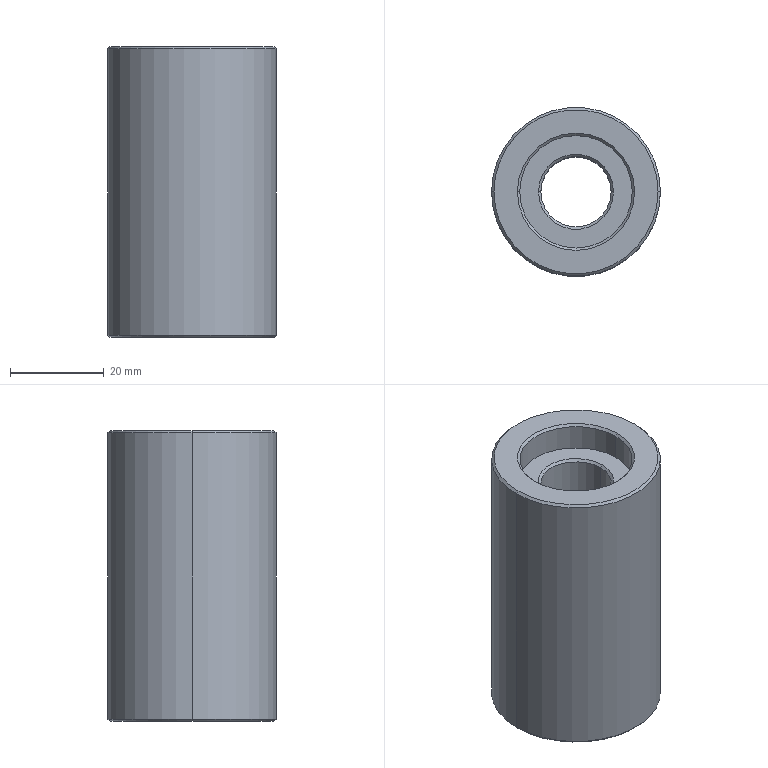Part | STEP file | 1 solid | 24 faces | box 36 x 36 x 62 mm | volume 48785 mm3 | cone 12 | cylinder 8 | plane 4 | commonest cylinder face diameters 24 x4 15 x2 36 x2
STEP:
#1=CARTESIAN_POINT('',(0.,0.,0.));
#2=DIRECTION('',(0.,0.,1.));
#3=DIRECTION('',(1.,0.,0.));
#4=AXIS2_PLACEMENT_3D('',#1,#2,#3);
#5=CARTESIAN_POINT('',(7.5,0.,55.5));
#6=VERTEX_POINT('',#5);
#7=CARTESIAN_POINT('',(8.,0.,56.));
#8=VERTEX_POINT('',#7);
#9=CARTESIAN_POINT('',(7.5,0.,55.5));
#10=DIRECTION('',(0.7071,0.,0.7071));
#11=VECTOR('',#10,1.);
#12=LINE('',#9,#11);
#13=CARTESIAN_POINT('',(0.,0.,55.5));
#14=DIRECTION('',(0.,0.,1.));
#15=DIRECTION('',(1.,0.,0.));
#16=AXIS2_PLACEMENT_3D('',#13,#14,#15);
#17=CONICAL_SURFACE('',#16,7.5,0.7854);
#18=CARTESIAN_POINT('',(6.283,0.));
#19=DIRECTION('',(0.,1.));
#20=VECTOR('',#19,1.);
#21=LINE('',#18,#20);
#22=(GEOMETRIC_REPRESENTATION_CONTEXT(2)PARAMETRIC_REPRESENTATION_CONTEXT()REPRESENTATION_CONTEXT('',''));
#23=DEFINITIONAL_REPRESENTATION('',(#21),#22);
#24=PCURVE('',#17,#23);
#25=CARTESIAN_POINT('',(0.,0.,55.5));
#26=DIRECTION('',(0.,0.,1.));
#27=DIRECTION('',(1.,0.,0.));
#28=AXIS2_PLACEMENT_3D('',#25,#26,#27);
#29=CONICAL_SURFACE('',#28,7.5,0.7854);
#30=CARTESIAN_POINT('',(0.,0.));
#31=DIRECTION('',(0.,1.));
#32=VECTOR('',#31,1.);
#33=LINE('',#30,#32);
#34=(GEOMETRIC_REPRESENTATION_CONTEXT(2)PARAMETRIC_REPRESENTATION_CONTEXT()REPRESENTATION_CONTEXT('',''));
#35=DEFINITIONAL_REPRESENTATION('',(#33),#34);
#36=PCURVE('',#29,#35);
#37=SURFACE_CURVE('',#12,(#24,#36),.PCURVE_S1.);
#38=EDGE_CURVE('',#6,#8,#37,.T.);
#39=ORIENTED_EDGE('',*,*,#38,.T.);
#40=CARTESIAN_POINT('',(-8.,0.,56.));
#41=VERTEX_POINT('',#40);
#42=CARTESIAN_POINT('',(0.,0.,56.));
#43=DIRECTION('',(0.,0.,-1.));
#44=DIRECTION('',(1.,0.,0.));
#45=AXIS2_PLACEMENT_3D('',#42,#43,#44);
#46=CIRCLE('',#45,8.);
#47=CARTESIAN_POINT('',(6.283,0.5));
#48=DIRECTION('',(-1.,0.));
#49=VECTOR('',#48,1.);
#50=LINE('',#47,#49);
#51=(GEOMETRIC_REPRESENTATION_CONTEXT(2)PARAMETRIC_REPRESENTATION_CONTEXT()REPRESENTATION_CONTEXT('',''));
#52=DEFINITIONAL_REPRESENTATION('',(#50),#51);
#53=PCURVE('',#17,#52);
#54=CARTESIAN_POINT('',(0.,0.,56.));
#55=DIRECTION('',(0.,0.,1.));
#56=DIRECTION('',(1.,0.,0.));
#57=AXIS2_PLACEMENT_3D('',#54,#55,#56);
#58=PLANE('',#57);
#59=CARTESIAN_POINT('',(8.,0.));
#60=CARTESIAN_POINT('',(8.,-13.856));
#61=CARTESIAN_POINT('',(-4.,-6.928));
#62=CARTESIAN_POINT('',(-16.,0.));
#63=CARTESIAN_POINT('',(-4.,6.928));
#64=CARTESIAN_POINT('',(8.,13.856));
#65=CARTESIAN_POINT('',(8.,0.));
#66=(BOUNDED_CURVE()B_SPLINE_CURVE(2,(#59,#60,#61,#62,#63,#64,#65),.UNSPECIFIED.,.T.,.F.)B_SPLINE_CURVE_WITH_KNOTS((1,2,2,2,2,1),(-2.094,0.,2.094,4.189,6.283,8.378),.UNSPECIFIED.)CURVE()GEOMETRIC_REPRESENTATION_ITEM()RATIONAL_B_SPLINE_CURVE((1.,0.5,1.,0.5,1.,0.5,1.))REPRESENTATION_ITEM(''));
#67=(GEOMETRIC_REPRESENTATION_CONTEXT(2)PARAMETRIC_REPRESENTATION_CONTEXT()REPRESENTATION_CONTEXT('',''));
#68=DEFINITIONAL_REPRESENTATION('',(#66),#67);
#69=PCURVE('',#58,#68);
#70=SURFACE_CURVE('',#46,(#53,#69),.PCURVE_S1.);
#71=EDGE_CURVE('',#8,#41,#70,.T.);
#72=ORIENTED_EDGE('',*,*,#71,.T.);
#73=CARTESIAN_POINT('',(-7.5,0.,55.5));
#74=VERTEX_POINT('',#73);
#75=CARTESIAN_POINT('',(-7.5,0.,55.5));
#76=DIRECTION('',(-0.7071,0.,0.7071));
#77=VECTOR('',#76,1.);
#78=LINE('',#75,#77);
#79=CARTESIAN_POINT('',(3.142,0.));
#80=DIRECTION('',(0.,1.));
#81=VECTOR('',#80,1.);
#82=LINE('',#79,#81);
#83=(GEOMETRIC_REPRESENTATION_CONTEXT(2)PARAMETRIC_REPRESENTATION_CONTEXT()REPRESENTATION_CONTEXT('',''));
#84=DEFINITIONAL_REPRESENTATION('',(#82),#83);
#85=PCURVE('',#17,#84);
#86=CARTESIAN_POINT('',(3.142,0.));
#87=DIRECTION('',(0.,1.));
#88=VECTOR('',#87,1.);
#89=LINE('',#86,#88);
#90=(GEOMETRIC_REPRESENTATION_CONTEXT(2)PARAMETRIC_REPRESENTATION_CONTEXT()REPRESENTATION_CONTEXT('',''));
#91=DEFINITIONAL_REPRESENTATION('',(#89),#90);
#92=PCURVE('',#29,#91);
#93=SURFACE_CURVE('',#78,(#85,#92),.PCURVE_S1.);
#94=EDGE_CURVE('',#74,#41,#93,.T.);
#95=ORIENTED_EDGE('',*,*,#94,.F.);
#96=CARTESIAN_POINT('',(0.,0.,55.5));
#97=DIRECTION('',(0.,0.,1.));
#98=DIRECTION('',(1.,0.,0.));
#99=AXIS2_PLACEMENT_3D('',#96,#97,#98);
#100=CIRCLE('',#99,7.5);
#101=CARTESIAN_POINT('',(0.,0.));
#102=DIRECTION('',(1.,0.));
#103=VECTOR('',#102,1.);
#104=LINE('',#101,#103);
#105=(GEOMETRIC_REPRESENTATION_CONTEXT(2)PARAMETRIC_REPRESENTATION_CONTEXT()REPRESENTATION_CONTEXT('',''));
#106=DEFINITIONAL_REPRESENTATION('',(#104),#105);
#107=PCURVE('',#17,#106);
#108=CARTESIAN_POINT('',(0.,0.,62.));
#109=DIRECTION('',(0.,0.,-1.));
#110=DIRECTION('',(-1.,0.,0.));
#111=AXIS2_PLACEMENT_3D('',#108,#109,#110);
#112=CYLINDRICAL_SURFACE('',#111,7.5);
#113=CARTESIAN_POINT('',(9.425,6.5));
#114=DIRECTION('',(-1.,0.));
#115=VECTOR('',#114,1.);
#116=LINE('',#113,#115);
#117=(GEOMETRIC_REPRESENTATION_CONTEXT(2)PARAMETRIC_REPRESENTATION_CONTEXT()REPRESENTATION_CONTEXT('',''));
#118=DEFINITIONAL_REPRESENTATION('',(#116),#117);
#119=PCURVE('',#112,#118);
#120=SURFACE_CURVE('',#100,(#107,#119),.PCURVE_S1.);
#121=EDGE_CURVE('',#74,#6,#120,.T.);
#122=ORIENTED_EDGE('',*,*,#121,.T.);
#123=EDGE_LOOP('',(#39,#72,#95,#122));
#124=FACE_BOUND('',#123,.F.);
#125=ADVANCED_FACE('',(#124),#17,.F.);
#126=CARTESIAN_POINT('',(12.,0.,61.5));
#127=VERTEX_POINT('',#126);
#128=CARTESIAN_POINT('',(12.5,0.,62.));
#129=VERTEX_POINT('',#128);
#130=CARTESIAN_POINT('',(12.,0.,61.5));
#131=DIRECTION('',(0.7071,0.,0.7071));
#132=VECTOR('',#131,1.);
#133=LINE('',#130,#132);
#134=CARTESIAN_POINT('',(0.,0.,61.5));
#135=DIRECTION('',(0.,0.,1.));
#136=DIRECTION('',(1.,0.,0.));
#137=AXIS2_PLACEMENT_3D('',#134,#135,#136);
#138=CONICAL_SURFACE('',#137,12.,0.7854);
#139=CARTESIAN_POINT('',(6.283,0.));
#140=DIRECTION('',(0.,1.));
#141=VECTOR('',#140,1.);
#142=LINE('',#139,#141);
#143=(GEOMETRIC_REPRESENTATION_CONTEXT(2)PARAMETRIC_REPRESENTATION_CONTEXT()REPRESENTATION_CONTEXT('',''));
#144=DEFINITIONAL_REPRESENTATION('',(#142),#143);
#145=PCURVE('',#138,#144);
#146=CARTESIAN_POINT('',(0.,0.,61.5));
#147=DIRECTION('',(0.,0.,1.));
#148=DIRECTION('',(1.,0.,0.));
#149=AXIS2_PLACEMENT_3D('',#146,#147,#148);
#150=CONICAL_SURFACE('',#149,12.,0.7854);
#151=CARTESIAN_POINT('',(0.,0.));
#152=DIRECTION('',(0.,1.));
#153=VECTOR('',#152,1.);
#154=LINE('',#151,#153);
#155=(GEOMETRIC_REPRESENTATION_CONTEXT(2)PARAMETRIC_REPRESENTATION_CONTEXT()REPRESENTATION_CONTEXT('',''));
#156=DEFINITIONAL_REPRESENTATION('',(#154),#155);
#157=PCURVE('',#150,#156);
#158=SURFACE_CURVE('',#133,(#145,#157),.PCURVE_S1.);
#159=EDGE_CURVE('',#127,#129,#158,.T.);
#160=ORIENTED_EDGE('',*,*,#159,.T.);
#161=CARTESIAN_POINT('',(-12.5,0.,62.));
#162=VERTEX_POINT('',#161);
#163=CARTESIAN_POINT('',(0.,0.,62.));
#164=DIRECTION('',(0.,0.,-1.));
#165=DIRECTION('',(1.,0.,0.));
#166=AXIS2_PLACEMENT_3D('',#163,#164,#165);
#167=CIRCLE('',#166,12.5);
#168=CARTESIAN_POINT('',(6.283,0.5));
#169=DIRECTION('',(-1.,0.));
#170=VECTOR('',#169,1.);
#171=LINE('',#168,#170);
#172=(GEOMETRIC_REPRESENTATION_CONTEXT(2)PARAMETRIC_REPRESENTATION_CONTEXT()REPRESENTATION_CONTEXT('',''));
#173=DEFINITIONAL_REPRESENTATION('',(#171),#172);
#174=PCURVE('',#138,#173);
#175=CARTESIAN_POINT('',(0.,0.,62.));
#176=DIRECTION('',(0.,0.,1.));
#177=DIRECTION('',(1.,0.,0.));
#178=AXIS2_PLACEMENT_3D('',#175,#176,#177);
#179=PLANE('',#178);
#180=CARTESIAN_POINT('',(12.5,0.));
#181=CARTESIAN_POINT('',(12.5,-21.651));
#182=CARTESIAN_POINT('',(-6.25,-10.825));
#183=CARTESIAN_POINT('',(-25.,0.));
#184=CARTESIAN_POINT('',(-6.25,10.825));
#185=CARTESIAN_POINT('',(12.5,21.651));
#186=CARTESIAN_POINT('',(12.5,0.));
#187=(BOUNDED_CURVE()B_SPLINE_CURVE(2,(#180,#181,#182,#183,#184,#185,#186),.UNSPECIFIED.,.T.,.F.)B_SPLINE_CURVE_WITH_KNOTS((1,2,2,2,2,1),(-2.094,0.,2.094,4.189,6.283,8.378),.UNSPECIFIED.)CURVE()GEOMETRIC_REPRESENTATION_ITEM()RATIONAL_B_SPLINE_CURVE((1.,0.5,1.,0.5,1.,0.5,1.))REPRESENTATION_ITEM(''));
#188=(GEOMETRIC_REPRESENTATION_CONTEXT(2)PARAMETRIC_REPRESENTATION_CONTEXT()REPRESENTATION_CONTEXT('',''));
#189=DEFINITIONAL_REPRESENTATION('',(#187),#188);
#190=PCURVE('',#179,#189);
#191=SURFACE_CURVE('',#167,(#174,#190),.PCURVE_S1.);
#192=EDGE_CURVE('',#129,#162,#191,.T.);
#193=ORIENTED_EDGE('',*,*,#192,.T.);
#194=CARTESIAN_POINT('',(-12.,0.,61.5));
#195=VERTEX_POINT('',#194);
#196=CARTESIAN_POINT('',(-12.,0.,61.5));
#197=DIRECTION('',(-0.7071,0.,0.7071));
#198=VECTOR('',#197,1.);
#199=LINE('',#196,#198);
#200=CARTESIAN_POINT('',(3.142,0.));
#201=DIRECTION('',(0.,1.));
#202=VECTOR('',#201,1.);
#203=LINE('',#200,#202);
#204=(GEOMETRIC_REPRESENTATION_CONTEXT(2)PARAMETRIC_REPRESENTATION_CONTEXT()REPRESENTATION_CONTEXT('',''));
#205=DEFINITIONAL_REPRESENTATION('',(#203),#204);
#206=PCURVE('',#138,#205);
#207=CARTESIAN_POINT('',(3.142,0.));
#208=DIRECTION('',(0.,1.));
#209=VECTOR('',#208,1.);
#210=LINE('',#207,#209);
#211=(GEOMETRIC_REPRESENTATION_CONTEXT(2)PARAMETRIC_REPRESENTATION_CONTEXT()REPRESENTATION_CONTEXT('',''));
#212=DEFINITIONAL_REPRESENTATION('',(#210),#211);
#213=PCURVE('',#150,#212);
#214=SURFACE_CURVE('',#199,(#206,#213),.PCURVE_S1.);
#215=EDGE_CURVE('',#195,#162,#214,.T.);
#216=ORIENTED_EDGE('',*,*,#215,.F.);
#217=CARTESIAN_POINT('',(0.,0.,61.5));
#218=DIRECTION('',(0.,0.,1.));
#219=DIRECTION('',(1.,0.,0.));
#220=AXIS2_PLACEMENT_3D('',#217,#218,#219);
#221=CIRCLE('',#220,12.);
#222=CARTESIAN_POINT('',(0.,0.));
#223=DIRECTION('',(1.,0.));
#224=VECTOR('',#223,1.);
#225=LINE('',#222,#224);
#226=(GEOMETRIC_REPRESENTATION_CONTEXT(2)PARAMETRIC_REPRESENTATION_CONTEXT()REPRESENTATION_CONTEXT('',''));
#227=DEFINITIONAL_REPRESENTATION('',(#225),#226);
#228=PCURVE('',#138,#227);
#229=CARTESIAN_POINT('',(0.,0.,56.));
#230=DIRECTION('',(0.,0.,1.));
#231=DIRECTION('',(1.,0.,0.));
#232=AXIS2_PLACEMENT_3D('',#229,#230,#231);
#233=CYLINDRICAL_SURFACE('',#232,12.);
#234=CARTESIAN_POINT('',(0.,5.5));
#235=DIRECTION('',(1.,0.));
#236=VECTOR('',#235,1.);
#237=LINE('',#234,#236);
#238=(GEOMETRIC_REPRESENTATION_CONTEXT(2)PARAMETRIC_REPRESENTATION_CONTEXT()REPRESENTATION_CONTEXT('',''));
#239=DEFINITIONAL_REPRESENTATION('',(#237),#238);
#240=PCURVE('',#233,#239);
#241=SURFACE_CURVE('',#221,(#228,#240),.PCURVE_S1.);
#242=EDGE_CURVE('',#195,#127,#241,.T.);
#243=ORIENTED_EDGE('',*,*,#242,.T.);
#244=EDGE_LOOP('',(#160,#193,#216,#243));
#245=FACE_BOUND('',#244,.F.);
#246=ADVANCED_FACE('',(#245),#138,.F.);
#247=CARTESIAN_POINT('',(-12.,0.,0.5));
#248=VERTEX_POINT('',#247);
#249=CARTESIAN_POINT('',(-12.5,0.,0.));
#250=VERTEX_POINT('',#249);
#251=CARTESIAN_POINT('',(-12.,0.,0.5));
#252=DIRECTION('',(-0.7071,0.,-0.7071));
#253=VECTOR('',#252,1.);
#254=LINE('',#251,#253);
#255=CARTESIAN_POINT('',(0.,0.,0.5));
#256=DIRECTION('',(0.,0.,-1.));
#257=DIRECTION('',(-1.,0.,0.));
#258=AXIS2_PLACEMENT_3D('',#255,#256,#257);
#259=CONICAL_SURFACE('',#258,12.,0.7854);
#260=CARTESIAN_POINT('',(6.283,0.));
#261=DIRECTION('',(0.,1.));
#262=VECTOR('',#261,1.);
#263=LINE('',#260,#262);
#264=(GEOMETRIC_REPRESENTATION_CONTEXT(2)PARAMETRIC_REPRESENTATION_CONTEXT()REPRESENTATION_CONTEXT('',''));
#265=DEFINITIONAL_REPRESENTATION('',(#263),#264);
#266=PCURVE('',#259,#265);
#267=CARTESIAN_POINT('',(0.,0.,0.5));
#268=DIRECTION('',(0.,0.,-1.));
#269=DIRECTION('',(-1.,0.,0.));
#270=AXIS2_PLACEMENT_3D('',#267,#268,#269);
#271=CONICAL_SURFACE('',#270,12.,0.7854);
#272=CARTESIAN_POINT('',(0.,0.));
#273=DIRECTION('',(0.,1.));
#274=VECTOR('',#273,1.);
#275=LINE('',#272,#274);
#276=(GEOMETRIC_REPRESENTATION_CONTEXT(2)PARAMETRIC_REPRESENTATION_CONTEXT()REPRESENTATION_CONTEXT('',''));
#277=DEFINITIONAL_REPRESENTATION('',(#275),#276);
#278=PCURVE('',#271,#277);
#279=SURFACE_CURVE('',#254,(#266,#278),.PCURVE_S1.);
#280=EDGE_CURVE('',#248,#250,#279,.T.);
#281=ORIENTED_EDGE('',*,*,#280,.T.);
#282=CARTESIAN_POINT('',(12.5,0.,0.));
#283=VERTEX_POINT('',#282);
#284=CARTESIAN_POINT('',(0.,0.,0.));
#285=DIRECTION('',(0.,0.,1.));
#286=DIRECTION('',(1.,0.,0.));
#287=AXIS2_PLACEMENT_3D('',#284,#285,#286);
#288=CIRCLE('',#287,12.5);
#289=CARTESIAN_POINT('',(9.425,0.5));
#290=DIRECTION('',(-1.,0.));
#291=VECTOR('',#290,1.);
#292=LINE('',#289,#291);
#293=(GEOMETRIC_REPRESENTATION_CONTEXT(2)PARAMETRIC_REPRESENTATION_CONTEXT()REPRESENTATION_CONTEXT('',''));
#294=DEFINITIONAL_REPRESENTATION('',(#292),#293);
#295=PCURVE('',#259,#294);
#296=CARTESIAN_POINT('',(0.,0.,0.));
#297=DIRECTION('',(0.,0.,1.));
#298=DIRECTION('',(1.,0.,0.));
#299=AXIS2_PLACEMENT_3D('',#296,#297,#298);
#300=PLANE('',#299);
#301=CARTESIAN_POINT('',(0.,0.));
#302=DIRECTION('',(1.,0.));
#303=AXIS2_PLACEMENT_2D('',#301,#302);
#304=CIRCLE('',#303,12.5);
#305=(GEOMETRIC_REPRESENTATION_CONTEXT(2)PARAMETRIC_REPRESENTATION_CONTEXT()REPRESENTATION_CONTEXT('',''));
#306=DEFINITIONAL_REPRESENTATION('',(#304),#305);
#307=PCURVE('',#300,#306);
#308=SURFACE_CURVE('',#288,(#295,#307),.PCURVE_S1.);
#309=EDGE_CURVE('',#250,#283,#308,.T.);
#310=ORIENTED_EDGE('',*,*,#309,.T.);
#311=CARTESIAN_POINT('',(12.,0.,0.5));
#312=VERTEX_POINT('',#311);
#313=CARTESIAN_POINT('',(12.,0.,0.5));
#314=DIRECTION('',(0.7071,0.,-0.7071));
#315=VECTOR('',#314,1.);
#316=LINE('',#313,#315);
#317=CARTESIAN_POINT('',(3.142,0.));
#318=DIRECTION('',(0.,1.));
#319=VECTOR('',#318,1.);
#320=LINE('',#317,#319);
#321=(GEOMETRIC_REPRESENTATION_CONTEXT(2)PARAMETRIC_REPRESENTATION_CONTEXT()REPRESENTATION_CONTEXT('',''));
#322=DEFINITIONAL_REPRESENTATION('',(#320),#321);
#323=PCURVE('',#259,#322);
#324=CARTESIAN_POINT('',(3.142,0.));
#325=DIRECTION('',(0.,1.));
#326=VECTOR('',#325,1.);
#327=LINE('',#324,#326);
#328=(GEOMETRIC_REPRESENTATION_CONTEXT(2)PARAMETRIC_REPRESENTATION_CONTEXT()REPRESENTATION_CONTEXT('',''));
#329=DEFINITIONAL_REPRESENTATION('',(#327),#328);
#330=PCURVE('',#271,#329);
#331=SURFACE_CURVE('',#316,(#323,#330),.PCURVE_S1.);
#332=EDGE_CURVE('',#312,#283,#331,.T.);
#333=ORIENTED_EDGE('',*,*,#332,.F.);
#334=CARTESIAN_POINT('',(0.,0.,0.5));
#335=DIRECTION('',(0.,0.,-1.));
#336=DIRECTION('',(1.,0.,0.));
#337=AXIS2_PLACEMENT_3D('',#334,#335,#336);
#338=CIRCLE('',#337,12.);
#339=CARTESIAN_POINT('',(3.142,0.));
#340=DIRECTION('',(1.,0.));
#341=VECTOR('',#340,1.);
#342=LINE('',#339,#341);
#343=(GEOMETRIC_REPRESENTATION_CONTEXT(2)PARAMETRIC_REPRESENTATION_CONTEXT()REPRESENTATION_CONTEXT('',''));
#344=DEFINITIONAL_REPRESENTATION('',(#342),#343);
#345=PCURVE('',#259,#344);
#346=CARTESIAN_POINT('',(0.,0.,6.));
#347=DIRECTION('',(0.,0.,-1.));
#348=DIRECTION('',(-1.,0.,0.));
#349=AXIS2_PLACEMENT_3D('',#346,#347,#348);
#350=CYLINDRICAL_SURFACE('',#349,12.);
#351=CARTESIAN_POINT('',(3.142,5.5));
#352=DIRECTION('',(1.,0.));
#353=VECTOR('',#352,1.);
#354=LINE('',#351,#353);
#355=(GEOMETRIC_REPRESENTATION_CONTEXT(2)PARAMETRIC_REPRESENTATION_CONTEXT()REPRESENTATION_CONTEXT('',''));
#356=DEFINITIONAL_REPRESENTATION('',(#354),#355);
#357=PCURVE('',#350,#356);
#358=SURFACE_CURVE('',#338,(#345,#357),.PCURVE_S1.);
#359=EDGE_CURVE('',#312,#248,#358,.T.);
#360=ORIENTED_EDGE('',*,*,#359,.T.);
#361=EDGE_LOOP('',(#281,#310,#333,#360));
#362=FACE_BOUND('',#361,.F.);
#363=ADVANCED_FACE('',(#362),#259,.F.);
#364=CARTESIAN_POINT('',(-17.5,0.,0.));
#365=VERTEX_POINT('',#364);
#366=CARTESIAN_POINT('',(17.5,0.,0.));
#367=VERTEX_POINT('',#366);
#368=CARTESIAN_POINT('',(0.,0.,0.));
#369=DIRECTION('',(0.,0.,-1.));
#370=DIRECTION('',(1.,0.,0.));
#371=AXIS2_PLACEMENT_3D('',#368,#369,#370);
#372=CIRCLE('',#371,17.5);
#373=CARTESIAN_POINT('',(0.,0.,0.5));
#374=DIRECTION('',(0.,0.,1.));
#375=DIRECTION('',(1.,0.,0.));
#376=AXIS2_PLACEMENT_3D('',#373,#374,#375);
#377=CONICAL_SURFACE('',#376,18.,0.7854);
#378=CARTESIAN_POINT('',(6.283,-0.5));
#379=DIRECTION('',(-1.,0.));
#380=VECTOR('',#379,1.);
#381=LINE('',#378,#380);
#382=(GEOMETRIC_REPRESENTATION_CONTEXT(2)PARAMETRIC_REPRESENTATION_CONTEXT()REPRESENTATION_CONTEXT('',''));
#383=DEFINITIONAL_REPRESENTATION('',(#381),#382);
#384=PCURVE('',#377,#383);
#385=CARTESIAN_POINT('',(17.5,0.));
#386=CARTESIAN_POINT('',(17.5,-30.311));
#387=CARTESIAN_POINT('',(-8.75,-15.155));
#388=CARTESIAN_POINT('',(-35.,0.));
#389=CARTESIAN_POINT('',(-8.75,15.155));
#390=CARTESIAN_POINT('',(17.5,30.311));
#391=CARTESIAN_POINT('',(17.5,0.));
#392=(BOUNDED_CURVE()B_SPLINE_CURVE(2,(#385,#386,#387,#388,#389,#390,#391),.UNSPECIFIED.,.T.,.F.)B_SPLINE_CURVE_WITH_KNOTS((1,2,2,2,2,1),(-2.094,0.,2.094,4.189,6.283,8.378),.UNSPECIFIED.)CURVE()GEOMETRIC_REPRESENTATION_ITEM()RATIONAL_B_SPLINE_CURVE((1.,0.5,1.,0.5,1.,0.5,1.))REPRESENTATION_ITEM(''));
#393=(GEOMETRIC_REPRESENTATION_CONTEXT(2)PARAMETRIC_REPRESENTATION_CONTEXT()REPRESENTATION_CONTEXT('',''));
#394=DEFINITIONAL_REPRESENTATION('',(#392),#393);
#395=PCURVE('',#300,#394);
#396=SURFACE_CURVE('',#372,(#384,#395),.PCURVE_S1.);
#397=EDGE_CURVE('',#365,#367,#396,.T.);
#398=ORIENTED_EDGE('',*,*,#397,.F.);
#399=CARTESIAN_POINT('',(-18.,0.,0.5));
#400=VERTEX_POINT('',#399);
#401=CARTESIAN_POINT('',(-18.,0.,0.5));
#402=DIRECTION('',(-0.7071,0.,0.7071));
#403=VECTOR('',#402,1.);
#404=LINE('',#401,#403);
#405=CARTESIAN_POINT('',(3.142,0.));
#406=DIRECTION('',(0.,1.));
#407=VECTOR('',#406,1.);
#408=LINE('',#405,#407);
#409=(GEOMETRIC_REPRESENTATION_CONTEXT(2)PARAMETRIC_REPRESENTATION_CONTEXT()REPRESENTATION_CONTEXT('',''));
#410=DEFINITIONAL_REPRESENTATION('',(#408),#409);
#411=PCURVE('',#377,#410);
#412=CARTESIAN_POINT('',(0.,0.,0.5));
#413=DIRECTION('',(0.,0.,1.));
#414=DIRECTION('',(1.,0.,0.));
#415=AXIS2_PLACEMENT_3D('',#412,#413,#414);
#416=CONICAL_SURFACE('',#415,18.,0.7854);
#417=CARTESIAN_POINT('',(3.142,0.));
#418=DIRECTION('',(0.,1.));
#419=VECTOR('',#418,1.);
#420=LINE('',#417,#419);
#421=(GEOMETRIC_REPRESENTATION_CONTEXT(2)PARAMETRIC_REPRESENTATION_CONTEXT()REPRESENTATION_CONTEXT('',''));
#422=DEFINITIONAL_REPRESENTATION('',(#420),#421);
#423=PCURVE('',#416,#422);
#424=SURFACE_CURVE('',#404,(#411,#423),.PCURVE_S1.);
#425=EDGE_CURVE('',#365,#400,#424,.T.);
#426=ORIENTED_EDGE('',*,*,#425,.T.);
#427=CARTESIAN_POINT('',(18.,0.,0.5));
#428=VERTEX_POINT('',#427);
#429=CARTESIAN_POINT('',(0.,0.,0.5));
#430=DIRECTION('',(0.,0.,1.));
#431=DIRECTION('',(1.,0.,0.));
#432=AXIS2_PLACEMENT_3D('',#429,#430,#431);
#433=CIRCLE('',#432,18.);
#434=CARTESIAN_POINT('',(0.,0.));
#435=DIRECTION('',(1.,0.));
#436=VECTOR('',#435,1.);
#437=LINE('',#434,#436);
#438=(GEOMETRIC_REPRESENTATION_CONTEXT(2)PARAMETRIC_REPRESENTATION_CONTEXT()REPRESENTATION_CONTEXT('',''));
#439=DEFINITIONAL_REPRESENTATION('',(#437),#438);
#440=PCURVE('',#377,#439);
#441=CARTESIAN_POINT('',(0.,0.,62.));
#442=DIRECTION('',(0.,0.,-1.));
#443=DIRECTION('',(-1.,0.,0.));
#444=AXIS2_PLACEMENT_3D('',#441,#442,#443);
#445=CYLINDRICAL_SURFACE('',#444,18.);
#446=CARTESIAN_POINT('',(3.142,61.5));
#447=DIRECTION('',(-1.,0.));
#448=VECTOR('',#447,1.);
#449=LINE('',#446,#448);
#450=(GEOMETRIC_REPRESENTATION_CONTEXT(2)PARAMETRIC_REPRESENTATION_CONTEXT()REPRESENTATION_CONTEXT('',''));
#451=DEFINITIONAL_REPRESENTATION('',(#449),#450);
#452=PCURVE('',#445,#451);
#453=SURFACE_CURVE('',#433,(#440,#452),.PCURVE_S1.);
#454=EDGE_CURVE('',#428,#400,#453,.T.);
#455=ORIENTED_EDGE('',*,*,#454,.F.);
#456=CARTESIAN_POINT('',(18.,0.,0.5));
#457=DIRECTION('',(0.7071,0.,0.7071));
#458=VECTOR('',#457,1.);
#459=LINE('',#456,#458);
#460=CARTESIAN_POINT('',(0.,0.));
#461=DIRECTION('',(0.,1.));
#462=VECTOR('',#461,1.);
#463=LINE('',#460,#462);
#464=(GEOMETRIC_REPRESENTATION_CONTEXT(2)PARAMETRIC_REPRESENTATION_CONTEXT()REPRESENTATION_CONTEXT('',''));
#465=DEFINITIONAL_REPRESENTATION('',(#463),#464);
#466=PCURVE('',#377,#465);
#467=CARTESIAN_POINT('',(6.283,0.));
#468=DIRECTION('',(0.,1.));
#469=VECTOR('',#468,1.);
#470=LINE('',#467,#469);
#471=(GEOMETRIC_REPRESENTATION_CONTEXT(2)PARAMETRIC_REPRESENTATION_CONTEXT()REPRESENTATION_CONTEXT('',''));
#472=DEFINITIONAL_REPRESENTATION('',(#470),#471);
#473=PCURVE('',#416,#472);
#474=SURFACE_CURVE('',#459,(#466,#473),.PCURVE_S1.);
#475=EDGE_CURVE('',#367,#428,#474,.T.);
#476=ORIENTED_EDGE('',*,*,#475,.F.);
#477=EDGE_LOOP('',(#398,#426,#455,#476));
#478=FACE_BOUND('',#477,.T.);
#479=ADVANCED_FACE('',(#478),#377,.T.);
#480=CARTESIAN_POINT('',(17.5,0.,62.));
#481=VERTEX_POINT('',#480);
#482=CARTESIAN_POINT('',(-17.5,0.,62.));
#483=VERTEX_POINT('',#482);
#484=CARTESIAN_POINT('',(0.,0.,62.));
#485=DIRECTION('',(0.,0.,1.));
#486=DIRECTION('',(1.,0.,0.));
#487=AXIS2_PLACEMENT_3D('',#484,#485,#486);
#488=CIRCLE('',#487,17.5);
#489=CARTESIAN_POINT('',(0.,0.,62.));
#490=DIRECTION('',(0.,0.,-1.));
#491=DIRECTION('',(-1.,0.,0.));
#492=AXIS2_PLACEMENT_3D('',#489,#490,#491);
#493=CONICAL_SURFACE('',#492,17.5,0.7854);
#494=CARTESIAN_POINT('',(3.142,0.));
#495=DIRECTION('',(-1.,0.));
#496=VECTOR('',#495,1.);
#497=LINE('',#494,#496);
#498=(GEOMETRIC_REPRESENTATION_CONTEXT(2)PARAMETRIC_REPRESENTATION_CONTEXT()REPRESENTATION_CONTEXT('',''));
#499=DEFINITIONAL_REPRESENTATION('',(#497),#498);
#500=PCURVE('',#493,#499);
#501=CARTESIAN_POINT('',(0.,0.));
#502=DIRECTION('',(1.,0.));
#503=AXIS2_PLACEMENT_2D('',#501,#502);
#504=CIRCLE('',#503,17.5);
#505=(GEOMETRIC_REPRESENTATION_CONTEXT(2)PARAMETRIC_REPRESENTATION_CONTEXT()REPRESENTATION_CONTEXT('',''));
#506=DEFINITIONAL_REPRESENTATION('',(#504),#505);
#507=PCURVE('',#179,#506);
#508=SURFACE_CURVE('',#488,(#500,#507),.PCURVE_S1.);
#509=EDGE_CURVE('',#481,#483,#508,.T.);
#510=ORIENTED_EDGE('',*,*,#509,.F.);
#511=CARTESIAN_POINT('',(18.,0.,61.5));
#512=VERTEX_POINT('',#511);
#513=CARTESIAN_POINT('',(17.5,0.,62.));
#514=DIRECTION('',(0.7071,0.,-0.7071));
#515=VECTOR('',#514,1.);
#516=LINE('',#513,#515);
#517=CARTESIAN_POINT('',(3.142,0.));
#518=DIRECTION('',(0.,1.));
#519=VECTOR('',#518,1.);
#520=LINE('',#517,#519);
#521=(GEOMETRIC_REPRESENTATION_CONTEXT(2)PARAMETRIC_REPRESENTATION_CONTEXT()REPRESENTATION_CONTEXT('',''));
#522=DEFINITIONAL_REPRESENTATION('',(#520),#521);
#523=PCURVE('',#493,#522);
#524=CARTESIAN_POINT('',(0.,0.,62.));
#525=DIRECTION('',(0.,0.,-1.));
#526=DIRECTION('',(-1.,0.,0.));
#527=AXIS2_PLACEMENT_3D('',#524,#525,#526);
#528=CONICAL_SURFACE('',#527,17.5,0.7854);
#529=CARTESIAN_POINT('',(3.142,0.));
#530=DIRECTION('',(0.,1.));
#531=VECTOR('',#530,1.);
#532=LINE('',#529,#531);
#533=(GEOMETRIC_REPRESENTATION_CONTEXT(2)PARAMETRIC_REPRESENTATION_CONTEXT()REPRESENTATION_CONTEXT('',''));
#534=DEFINITIONAL_REPRESENTATION('',(#532),#533);
#535=PCURVE('',#528,#534);
#536=SURFACE_CURVE('',#516,(#523,#535),.PCURVE_S1.);
#537=EDGE_CURVE('',#481,#512,#536,.T.);
#538=ORIENTED_EDGE('',*,*,#537,.T.);
#539=CARTESIAN_POINT('',(-18.,0.,61.5));
#540=VERTEX_POINT('',#539);
#541=CARTESIAN_POINT('',(0.,0.,61.5));
#542=DIRECTION('',(0.,0.,-1.));
#543=DIRECTION('',(1.,0.,0.));
#544=AXIS2_PLACEMENT_3D('',#541,#542,#543);
#545=CIRCLE('',#544,18.);
#546=CARTESIAN_POINT('',(-3.142,0.5));
#547=DIRECTION('',(1.,0.));
#548=VECTOR('',#547,1.);
#549=LINE('',#546,#548);
#550=(GEOMETRIC_REPRESENTATION_CONTEXT(2)PARAMETRIC_REPRESENTATION_CONTEXT()REPRESENTATION_CONTEXT('',''));
#551=DEFINITIONAL_REPRESENTATION('',(#549),#550);
#552=PCURVE('',#493,#551);
#553=CARTESIAN_POINT('',(-3.142,0.5));
#554=DIRECTION('',(1.,0.));
#555=VECTOR('',#554,1.);
#556=LINE('',#553,#555);
#557=(GEOMETRIC_REPRESENTATION_CONTEXT(2)PARAMETRIC_REPRESENTATION_CONTEXT()REPRESENTATION_CONTEXT('',''));
#558=DEFINITIONAL_REPRESENTATION('',(#556),#557);
#559=PCURVE('',#445,#558);
#560=SURFACE_CURVE('',#545,(#552,#559),.PCURVE_S1.);
#561=EDGE_CURVE('',#540,#512,#560,.T.);
#562=ORIENTED_EDGE('',*,*,#561,.F.);
#563=CARTESIAN_POINT('',(-17.5,0.,62.));
#564=DIRECTION('',(-0.7071,0.,-0.7071));
#565=VECTOR('',#564,1.);
#566=LINE('',#563,#565);
#567=CARTESIAN_POINT('',(0.,0.));
#568=DIRECTION('',(0.,1.));
#569=VECTOR('',#568,1.);
#570=LINE('',#567,#569);
#571=(GEOMETRIC_REPRESENTATION_CONTEXT(2)PARAMETRIC_REPRESENTATION_CONTEXT()REPRESENTATION_CONTEXT('',''));
#572=DEFINITIONAL_REPRESENTATION('',(#570),#571);
#573=PCURVE('',#493,#572);
#574=CARTESIAN_POINT('',(6.283,0.));
#575=DIRECTION('',(0.,1.));
#576=VECTOR('',#575,1.);
#577=LINE('',#574,#576);
#578=(GEOMETRIC_REPRESENTATION_CONTEXT(2)PARAMETRIC_REPRESENTATION_CONTEXT()REPRESENTATION_CONTEXT('',''));
#579=DEFINITIONAL_REPRESENTATION('',(#577),#578);
#580=PCURVE('',#528,#579);
#581=SURFACE_CURVE('',#566,(#573,#580),.PCURVE_S1.);
#582=EDGE_CURVE('',#483,#540,#581,.T.);
#583=ORIENTED_EDGE('',*,*,#582,.F.);
#584=EDGE_LOOP('',(#510,#538,#562,#583));
#585=FACE_BOUND('',#584,.T.);
#586=ADVANCED_FACE('',(#585),#493,.T.);
#587=CARTESIAN_POINT('',(-7.5,0.,6.5));
#588=VERTEX_POINT('',#587);
#589=CARTESIAN_POINT('',(-8.,0.,6.));
#590=VERTEX_POINT('',#589);
#591=CARTESIAN_POINT('',(-7.5,0.,6.5));
#592=DIRECTION('',(-0.7071,0.,-0.7071));
#593=VECTOR('',#592,1.);
#594=LINE('',#591,#593);
#595=CARTESIAN_POINT('',(0.,0.,6.5));
#596=DIRECTION('',(0.,0.,-1.));
#597=DIRECTION('',(-1.,0.,0.));
#598=AXIS2_PLACEMENT_3D('',#595,#596,#597);
#599=CONICAL_SURFACE('',#598,7.5,0.7854);
#600=CARTESIAN_POINT('',(6.283,0.));
#601=DIRECTION('',(0.,1.));
#602=VECTOR('',#601,1.);
#603=LINE('',#600,#602);
#604=(GEOMETRIC_REPRESENTATION_CONTEXT(2)PARAMETRIC_REPRESENTATION_CONTEXT()REPRESENTATION_CONTEXT('',''));
#605=DEFINITIONAL_REPRESENTATION('',(#603),#604);
#606=PCURVE('',#599,#605);
#607=CARTESIAN_POINT('',(0.,0.,6.5));
#608=DIRECTION('',(0.,0.,-1.));
#609=DIRECTION('',(-1.,0.,0.));
#610=AXIS2_PLACEMENT_3D('',#607,#608,#609);
#611=CONICAL_SURFACE('',#610,7.5,0.7854);
#612=CARTESIAN_POINT('',(0.,0.));
#613=DIRECTION('',(0.,1.));
#614=VECTOR('',#613,1.);
#615=LINE('',#612,#614);
#616=(GEOMETRIC_REPRESENTATION_CONTEXT(2)PARAMETRIC_REPRESENTATION_CONTEXT()REPRESENTATION_CONTEXT('',''));
#617=DEFINITIONAL_REPRESENTATION('',(#615),#616);
#618=PCURVE('',#611,#617);
#619=SURFACE_CURVE('',#594,(#606,#618),.PCURVE_S1.);
#620=EDGE_CURVE('',#588,#590,#619,.T.);
#621=ORIENTED_EDGE('',*,*,#620,.T.);
#622=CARTESIAN_POINT('',(8.,0.,6.));
#623=VERTEX_POINT('',#622);
#624=CARTESIAN_POINT('',(0.,0.,6.));
#625=DIRECTION('',(0.,0.,1.));
#626=DIRECTION('',(-1.,0.,0.));
#627=AXIS2_PLACEMENT_3D('',#624,#625,#626);
#628=CIRCLE('',#627,8.);
#629=CARTESIAN_POINT('',(6.283,0.5));
#630=DIRECTION('',(-1.,0.));
#631=VECTOR('',#630,1.);
#632=LINE('',#629,#631);
#633=(GEOMETRIC_REPRESENTATION_CONTEXT(2)PARAMETRIC_REPRESENTATION_CONTEXT()REPRESENTATION_CONTEXT('',''));
#634=DEFINITIONAL_REPRESENTATION('',(#632),#633);
#635=PCURVE('',#599,#634);
#636=CARTESIAN_POINT('',(0.,0.,6.));
#637=DIRECTION('',(0.,0.,-1.));
#638=DIRECTION('',(-1.,0.,0.));
#639=AXIS2_PLACEMENT_3D('',#636,#637,#638);
#640=PLANE('',#639);
#641=CARTESIAN_POINT('',(8.,0.));
#642=CARTESIAN_POINT('',(8.,-13.856));
#643=CARTESIAN_POINT('',(-4.,-6.928));
#644=CARTESIAN_POINT('',(-16.,0.));
#645=CARTESIAN_POINT('',(-4.,6.928));
#646=CARTESIAN_POINT('',(8.,13.856));
#647=CARTESIAN_POINT('',(8.,0.));
#648=(BOUNDED_CURVE()B_SPLINE_CURVE(2,(#641,#642,#643,#644,#645,#646,#647),.UNSPECIFIED.,.T.,.F.)B_SPLINE_CURVE_WITH_KNOTS((1,2,2,2,2,1),(-2.094,0.,2.094,4.189,6.283,8.378),.UNSPECIFIED.)CURVE()GEOMETRIC_REPRESENTATION_ITEM()RATIONAL_B_SPLINE_CURVE((1.,0.5,1.,0.5,1.,0.5,1.))REPRESENTATION_ITEM(''));
#649=(GEOMETRIC_REPRESENTATION_CONTEXT(2)PARAMETRIC_REPRESENTATION_CONTEXT()REPRESENTATION_CONTEXT('',''));
#650=DEFINITIONAL_REPRESENTATION('',(#648),#649);
#651=PCURVE('',#640,#650);
#652=SURFACE_CURVE('',#628,(#635,#651),.PCURVE_S1.);
#653=EDGE_CURVE('',#590,#623,#652,.T.);
#654=ORIENTED_EDGE('',*,*,#653,.T.);
#655=CARTESIAN_POINT('',(7.5,0.,6.5));
#656=VERTEX_POINT('',#655);
#657=CARTESIAN_POINT('',(7.5,0.,6.5));
#658=DIRECTION('',(0.7071,0.,-0.7071));
#659=VECTOR('',#658,1.);
#660=LINE('',#657,#659);
#661=CARTESIAN_POINT('',(3.142,0.));
#662=DIRECTION('',(0.,1.));
#663=VECTOR('',#662,1.);
#664=LINE('',#661,#663);
#665=(GEOMETRIC_REPRESENTATION_CONTEXT(2)PARAMETRIC_REPRESENTATION_CONTEXT()REPRESENTATION_CONTEXT('',''));
#666=DEFINITIONAL_REPRESENTATION('',(#664),#665);
#667=PCURVE('',#599,#666);
#668=CARTESIAN_POINT('',(3.142,0.));
#669=DIRECTION('',(0.,1.));
#670=VECTOR('',#669,1.);
#671=LINE('',#668,#670);
#672=(GEOMETRIC_REPRESENTATION_CONTEXT(2)PARAMETRIC_REPRESENTATION_CONTEXT()REPRESENTATION_CONTEXT('',''));
#673=DEFINITIONAL_REPRESENTATION('',(#671),#672);
#674=PCURVE('',#611,#673);
#675=SURFACE_CURVE('',#660,(#667,#674),.PCURVE_S1.);
#676=EDGE_CURVE('',#656,#623,#675,.T.);
#677=ORIENTED_EDGE('',*,*,#676,.F.);
#678=CARTESIAN_POINT('',(0.,0.,6.5));
#679=DIRECTION('',(0.,0.,-1.));
#680=DIRECTION('',(-1.,0.,0.));
#681=AXIS2_PLACEMENT_3D('',#678,#679,#680);
#682=CIRCLE('',#681,7.5);
#683=CARTESIAN_POINT('',(0.,0.));
#684=DIRECTION('',(1.,0.));
#685=VECTOR('',#684,1.);
#686=LINE('',#683,#685);
#687=(GEOMETRIC_REPRESENTATION_CONTEXT(2)PARAMETRIC_REPRESENTATION_CONTEXT()REPRESENTATION_CONTEXT('',''));
#688=DEFINITIONAL_REPRESENTATION('',(#686),#687);
#689=PCURVE('',#599,#688);
#690=CARTESIAN_POINT('',(0.,55.5));
#691=DIRECTION('',(1.,0.));
#692=VECTOR('',#691,1.);
#693=LINE('',#690,#692);
#694=(GEOMETRIC_REPRESENTATION_CONTEXT(2)PARAMETRIC_REPRESENTATION_CONTEXT()REPRESENTATION_CONTEXT('',''));
#695=DEFINITIONAL_REPRESENTATION('',(#693),#694);
#696=PCURVE('',#112,#695);
#697=SURFACE_CURVE('',#682,(#689,#696),.PCURVE_S1.);
#698=EDGE_CURVE('',#656,#588,#697,.T.);
#699=ORIENTED_EDGE('',*,*,#698,.T.);
#700=EDGE_LOOP('',(#621,#654,#677,#699));
#701=FACE_BOUND('',#700,.F.);
#702=ADVANCED_FACE('',(#701),#599,.F.);
#703=CARTESIAN_POINT('',(-7.5,0.,62.));
#704=DIRECTION('',(0.,0.,-1.));
#705=VECTOR('',#704,1.);
#706=LINE('',#703,#705);
#707=CARTESIAN_POINT('',(6.283,0.));
#708=DIRECTION('',(0.,1.));
#709=VECTOR('',#708,1.);
#710=LINE('',#707,#709);
#711=(GEOMETRIC_REPRESENTATION_CONTEXT(2)PARAMETRIC_REPRESENTATION_CONTEXT()REPRESENTATION_CONTEXT('',''));
#712=DEFINITIONAL_REPRESENTATION('',(#710),#711);
#713=PCURVE('',#112,#712);
#714=CARTESIAN_POINT('',(0.,0.,62.));
#715=DIRECTION('',(0.,0.,-1.));
#716=DIRECTION('',(-1.,0.,0.));
#717=AXIS2_PLACEMENT_3D('',#714,#715,#716);
#718=CYLINDRICAL_SURFACE('',#717,7.5);
#719=CARTESIAN_POINT('',(0.,0.));
#720=DIRECTION('',(0.,1.));
#721=VECTOR('',#720,1.);
#722=LINE('',#719,#721);
#723=(GEOMETRIC_REPRESENTATION_CONTEXT(2)PARAMETRIC_REPRESENTATION_CONTEXT()REPRESENTATION_CONTEXT('',''));
#724=DEFINITIONAL_REPRESENTATION('',(#722),#723);
#725=PCURVE('',#718,#724);
#726=SURFACE_CURVE('',#706,(#713,#725),.PCURVE_S1.);
#727=EDGE_CURVE('',#74,#588,#726,.T.);
#728=ORIENTED_EDGE('',*,*,#727,.T.);
#729=ORIENTED_EDGE('',*,*,#698,.F.);
#730=CARTESIAN_POINT('',(7.5,0.,62.));
#731=DIRECTION('',(0.,0.,-1.));
#732=VECTOR('',#731,1.);
#733=LINE('',#730,#732);
#734=CARTESIAN_POINT('',(3.142,0.));
#735=DIRECTION('',(0.,1.));
#736=VECTOR('',#735,1.);
#737=LINE('',#734,#736);
#738=(GEOMETRIC_REPRESENTATION_CONTEXT(2)PARAMETRIC_REPRESENTATION_CONTEXT()REPRESENTATION_CONTEXT('',''));
#739=DEFINITIONAL_REPRESENTATION('',(#737),#738);
#740=PCURVE('',#112,#739);
#741=CARTESIAN_POINT('',(3.142,0.));
#742=DIRECTION('',(0.,1.));
#743=VECTOR('',#742,1.);
#744=LINE('',#741,#743);
#745=(GEOMETRIC_REPRESENTATION_CONTEXT(2)PARAMETRIC_REPRESENTATION_CONTEXT()REPRESENTATION_CONTEXT('',''));
#746=DEFINITIONAL_REPRESENTATION('',(#744),#745);
#747=PCURVE('',#718,#746);
#748=SURFACE_CURVE('',#733,(#740,#747),.PCURVE_S1.);
#749=EDGE_CURVE('',#6,#656,#748,.T.);
#750=ORIENTED_EDGE('',*,*,#749,.F.);
#751=ORIENTED_EDGE('',*,*,#121,.F.);
#752=EDGE_LOOP('',(#728,#729,#750,#751));
#753=FACE_BOUND('',#752,.F.);
#754=ADVANCED_FACE('',(#753),#112,.F.);
#755=CARTESIAN_POINT('',(-12.,0.,6.));
#756=VERTEX_POINT('',#755);
#757=CARTESIAN_POINT('',(-12.,0.,6.));
#758=DIRECTION('',(0.,0.,-1.));
#759=VECTOR('',#758,1.);
#760=LINE('',#757,#759);
#761=CARTESIAN_POINT('',(6.283,0.));
#762=DIRECTION('',(0.,1.));
#763=VECTOR('',#762,1.);
#764=LINE('',#761,#763);
#765=(GEOMETRIC_REPRESENTATION_CONTEXT(2)PARAMETRIC_REPRESENTATION_CONTEXT()REPRESENTATION_CONTEXT('',''));
#766=DEFINITIONAL_REPRESENTATION('',(#764),#765);
#767=PCURVE('',#350,#766);
#768=CARTESIAN_POINT('',(0.,0.,6.));
#769=DIRECTION('',(0.,0.,-1.));
#770=DIRECTION('',(-1.,0.,0.));
#771=AXIS2_PLACEMENT_3D('',#768,#769,#770);
#772=CYLINDRICAL_SURFACE('',#771,12.);
#773=CARTESIAN_POINT('',(0.,0.));
#774=DIRECTION('',(0.,1.));
#775=VECTOR('',#774,1.);
#776=LINE('',#773,#775);
#777=(GEOMETRIC_REPRESENTATION_CONTEXT(2)PARAMETRIC_REPRESENTATION_CONTEXT()REPRESENTATION_CONTEXT('',''));
#778=DEFINITIONAL_REPRESENTATION('',(#776),#777);
#779=PCURVE('',#772,#778);
#780=SURFACE_CURVE('',#760,(#767,#779),.PCURVE_S1.);
#781=EDGE_CURVE('',#756,#248,#780,.T.);
#782=ORIENTED_EDGE('',*,*,#781,.T.);
#783=ORIENTED_EDGE('',*,*,#359,.F.);
#784=CARTESIAN_POINT('',(12.,0.,6.));
#785=VERTEX_POINT('',#784);
#786=CARTESIAN_POINT('',(12.,0.,6.));
#787=DIRECTION('',(0.,0.,-1.));
#788=VECTOR('',#787,1.);
#789=LINE('',#786,#788);
#790=CARTESIAN_POINT('',(3.142,0.));
#791=DIRECTION('',(0.,1.));
#792=VECTOR('',#791,1.);
#793=LINE('',#790,#792);
#794=(GEOMETRIC_REPRESENTATION_CONTEXT(2)PARAMETRIC_REPRESENTATION_CONTEXT()REPRESENTATION_CONTEXT('',''));
#795=DEFINITIONAL_REPRESENTATION('',(#793),#794);
#796=PCURVE('',#350,#795);
#797=CARTESIAN_POINT('',(3.142,0.));
#798=DIRECTION('',(0.,1.));
#799=VECTOR('',#798,1.);
#800=LINE('',#797,#799);
#801=(GEOMETRIC_REPRESENTATION_CONTEXT(2)PARAMETRIC_REPRESENTATION_CONTEXT()REPRESENTATION_CONTEXT('',''));
#802=DEFINITIONAL_REPRESENTATION('',(#800),#801);
#803=PCURVE('',#772,#802);
#804=SURFACE_CURVE('',#789,(#796,#803),.PCURVE_S1.);
#805=EDGE_CURVE('',#785,#312,#804,.T.);
#806=ORIENTED_EDGE('',*,*,#805,.F.);
#807=CARTESIAN_POINT('',(0.,0.,6.));
#808=DIRECTION('',(0.,0.,-1.));
#809=DIRECTION('',(-1.,0.,0.));
#810=AXIS2_PLACEMENT_3D('',#807,#808,#809);
#811=CIRCLE('',#810,12.);
#812=CARTESIAN_POINT('',(0.,0.));
#813=DIRECTION('',(1.,0.));
#814=VECTOR('',#813,1.);
#815=LINE('',#812,#814);
#816=(GEOMETRIC_REPRESENTATION_CONTEXT(2)PARAMETRIC_REPRESENTATION_CONTEXT()REPRESENTATION_CONTEXT('',''));
#817=DEFINITIONAL_REPRESENTATION('',(#815),#816);
#818=PCURVE('',#350,#817);
#819=CARTESIAN_POINT('',(0.,0.));
#820=DIRECTION('',(1.,0.));
#821=AXIS2_PLACEMENT_2D('',#819,#820);
#822=CIRCLE('',#821,12.);
#823=(GEOMETRIC_REPRESENTATION_CONTEXT(2)PARAMETRIC_REPRESENTATION_CONTEXT()REPRESENTATION_CONTEXT('',''));
#824=DEFINITIONAL_REPRESENTATION('',(#822),#823);
#825=PCURVE('',#640,#824);
#826=SURFACE_CURVE('',#811,(#818,#825),.PCURVE_S1.);
#827=EDGE_CURVE('',#785,#756,#826,.T.);
#828=ORIENTED_EDGE('',*,*,#827,.T.);
#829=EDGE_LOOP('',(#782,#783,#806,#828));
#830=FACE_BOUND('',#829,.F.);
#831=ADVANCED_FACE('',(#830),#350,.F.);
#832=CARTESIAN_POINT('',(12.,0.,56.));
#833=VERTEX_POINT('',#832);
#834=CARTESIAN_POINT('',(12.,0.,56.));
#835=DIRECTION('',(0.,0.,1.));
#836=VECTOR('',#835,1.);
#837=LINE('',#834,#836);
#838=CARTESIAN_POINT('',(6.283,0.));
#839=DIRECTION('',(0.,1.));
#840=VECTOR('',#839,1.);
#841=LINE('',#838,#840);
#842=(GEOMETRIC_REPRESENTATION_CONTEXT(2)PARAMETRIC_REPRESENTATION_CONTEXT()REPRESENTATION_CONTEXT('',''));
#843=DEFINITIONAL_REPRESENTATION('',(#841),#842);
#844=PCURVE('',#233,#843);
#845=CARTESIAN_POINT('',(0.,0.,56.));
#846=DIRECTION('',(0.,0.,1.));
#847=DIRECTION('',(1.,0.,0.));
#848=AXIS2_PLACEMENT_3D('',#845,#846,#847);
#849=CYLINDRICAL_SURFACE('',#848,12.);
#850=CARTESIAN_POINT('',(0.,0.));
#851=DIRECTION('',(0.,1.));
#852=VECTOR('',#851,1.);
#853=LINE('',#850,#852);
#854=(GEOMETRIC_REPRESENTATION_CONTEXT(2)PARAMETRIC_REPRESENTATION_CONTEXT()REPRESENTATION_CONTEXT('',''));
#855=DEFINITIONAL_REPRESENTATION('',(#853),#854);
#856=PCURVE('',#849,#855);
#857=SURFACE_CURVE('',#837,(#844,#856),.PCURVE_S1.);
#858=EDGE_CURVE('',#833,#127,#857,.T.);
#859=ORIENTED_EDGE('',*,*,#858,.T.);
#860=ORIENTED_EDGE('',*,*,#242,.F.);
#861=CARTESIAN_POINT('',(-12.,0.,56.));
#862=VERTEX_POINT('',#861);
#863=CARTESIAN_POINT('',(-12.,0.,56.));
#864=DIRECTION('',(0.,0.,1.));
#865=VECTOR('',#864,1.);
#866=LINE('',#863,#865);
#867=CARTESIAN_POINT('',(3.142,0.));
#868=DIRECTION('',(0.,1.));
#869=VECTOR('',#868,1.);
#870=LINE('',#867,#869);
#871=(GEOMETRIC_REPRESENTATION_CONTEXT(2)PARAMETRIC_REPRESENTATION_CONTEXT()REPRESENTATION_CONTEXT('',''));
#872=DEFINITIONAL_REPRESENTATION('',(#870),#871);
#873=PCURVE('',#233,#872);
#874=CARTESIAN_POINT('',(3.142,0.));
#875=DIRECTION('',(0.,1.));
#876=VECTOR('',#875,1.);
#877=LINE('',#874,#876);
#878=(GEOMETRIC_REPRESENTATION_CONTEXT(2)PARAMETRIC_REPRESENTATION_CONTEXT()REPRESENTATION_CONTEXT('',''));
#879=DEFINITIONAL_REPRESENTATION('',(#877),#878);
#880=PCURVE('',#849,#879);
#881=SURFACE_CURVE('',#866,(#873,#880),.PCURVE_S1.);
#882=EDGE_CURVE('',#862,#195,#881,.T.);
#883=ORIENTED_EDGE('',*,*,#882,.F.);
#884=CARTESIAN_POINT('',(0.,0.,56.));
#885=DIRECTION('',(0.,0.,1.));
#886=DIRECTION('',(1.,0.,0.));
#887=AXIS2_PLACEMENT_3D('',#884,#885,#886);
#888=CIRCLE('',#887,12.);
#889=CARTESIAN_POINT('',(0.,0.));
#890=DIRECTION('',(1.,0.));
#891=VECTOR('',#890,1.);
#892=LINE('',#889,#891);
#893=(GEOMETRIC_REPRESENTATION_CONTEXT(2)PARAMETRIC_REPRESENTATION_CONTEXT()REPRESENTATION_CONTEXT('',''));
#894=DEFINITIONAL_REPRESENTATION('',(#892),#893);
#895=PCURVE('',#233,#894);
#896=CARTESIAN_POINT('',(0.,0.));
#897=DIRECTION('',(1.,0.));
#898=AXIS2_PLACEMENT_2D('',#896,#897);
#899=CIRCLE('',#898,12.);
#900=(GEOMETRIC_REPRESENTATION_CONTEXT(2)PARAMETRIC_REPRESENTATION_CONTEXT()REPRESENTATION_CONTEXT('',''));
#901=DEFINITIONAL_REPRESENTATION('',(#899),#900);
#902=PCURVE('',#58,#901);
#903=SURFACE_CURVE('',#888,(#895,#902),.PCURVE_S1.);
#904=EDGE_CURVE('',#862,#833,#903,.T.);
#905=ORIENTED_EDGE('',*,*,#904,.T.);
#906=EDGE_LOOP('',(#859,#860,#883,#905));
#907=FACE_BOUND('',#906,.F.);
#908=ADVANCED_FACE('',(#907),#233,.F.);
#909=ORIENTED_EDGE('',*,*,#561,.T.);
#910=CARTESIAN_POINT('',(18.,0.,62.));
#911=DIRECTION('',(0.,0.,-1.));
#912=VECTOR('',#911,1.);
#913=LINE('',#910,#912);
#914=CARTESIAN_POINT('',(3.142,0.));
#915=DIRECTION('',(0.,1.));
#916=VECTOR('',#915,1.);
#917=LINE('',#914,#916);
#918=(GEOMETRIC_REPRESENTATION_CONTEXT(2)PARAMETRIC_REPRESENTATION_CONTEXT()REPRESENTATION_CONTEXT('',''));
#919=DEFINITIONAL_REPRESENTATION('',(#917),#918);
#920=PCURVE('',#445,#919);
#921=CARTESIAN_POINT('',(0.,0.,62.));
#922=DIRECTION('',(0.,0.,-1.));
#923=DIRECTION('',(-1.,0.,0.));
#924=AXIS2_PLACEMENT_3D('',#921,#922,#923);
#925=CYLINDRICAL_SURFACE('',#924,18.);
#926=CARTESIAN_POINT('',(3.142,0.));
#927=DIRECTION('',(0.,1.));
#928=VECTOR('',#927,1.);
#929=LINE('',#926,#928);
#930=(GEOMETRIC_REPRESENTATION_CONTEXT(2)PARAMETRIC_REPRESENTATION_CONTEXT()REPRESENTATION_CONTEXT('',''));
#931=DEFINITIONAL_REPRESENTATION('',(#929),#930);
#932=PCURVE('',#925,#931);
#933=SURFACE_CURVE('',#913,(#920,#932),.PCURVE_S1.);
#934=EDGE_CURVE('',#512,#428,#933,.T.);
#935=ORIENTED_EDGE('',*,*,#934,.T.);
#936=ORIENTED_EDGE('',*,*,#454,.T.);
#937=CARTESIAN_POINT('',(-18.,0.,62.));
#938=DIRECTION('',(0.,0.,-1.));
#939=VECTOR('',#938,1.);
#940=LINE('',#937,#939);
#941=CARTESIAN_POINT('',(0.,0.));
#942=DIRECTION('',(0.,1.));
#943=VECTOR('',#942,1.);
#944=LINE('',#941,#943);
#945=(GEOMETRIC_REPRESENTATION_CONTEXT(2)PARAMETRIC_REPRESENTATION_CONTEXT()REPRESENTATION_CONTEXT('',''));
#946=DEFINITIONAL_REPRESENTATION('',(#944),#945);
#947=PCURVE('',#445,#946);
#948=CARTESIAN_POINT('',(6.283,0.));
#949=DIRECTION('',(0.,1.));
#950=VECTOR('',#949,1.);
#951=LINE('',#948,#950);
#952=(GEOMETRIC_REPRESENTATION_CONTEXT(2)PARAMETRIC_REPRESENTATION_CONTEXT()REPRESENTATION_CONTEXT('',''));
#953=DEFINITIONAL_REPRESENTATION('',(#951),#952);
#954=PCURVE('',#925,#953);
#955=SURFACE_CURVE('',#940,(#947,#954),.PCURVE_S1.);
#956=EDGE_CURVE('',#540,#400,#955,.T.);
#957=ORIENTED_EDGE('',*,*,#956,.F.);
#958=EDGE_LOOP('',(#909,#935,#936,#957));
#959=FACE_BOUND('',#958,.T.);
#960=ADVANCED_FACE('',(#959),#445,.T.);
#961=ORIENTED_EDGE('',*,*,#934,.F.);
#962=CARTESIAN_POINT('',(0.,0.,61.5));
#963=DIRECTION('',(0.,0.,-1.));
#964=DIRECTION('',(1.,0.,0.));
#965=AXIS2_PLACEMENT_3D('',#962,#963,#964);
#966=CIRCLE('',#965,18.);
#967=CARTESIAN_POINT('',(3.142,0.5));
#968=DIRECTION('',(1.,0.));
#969=VECTOR('',#968,1.);
#970=LINE('',#967,#969);
#971=(GEOMETRIC_REPRESENTATION_CONTEXT(2)PARAMETRIC_REPRESENTATION_CONTEXT()REPRESENTATION_CONTEXT('',''));
#972=DEFINITIONAL_REPRESENTATION('',(#970),#971);
#973=PCURVE('',#925,#972);
#974=CARTESIAN_POINT('',(3.142,0.5));
#975=DIRECTION('',(1.,0.));
#976=VECTOR('',#975,1.);
#977=LINE('',#974,#976);
#978=(GEOMETRIC_REPRESENTATION_CONTEXT(2)PARAMETRIC_REPRESENTATION_CONTEXT()REPRESENTATION_CONTEXT('',''));
#979=DEFINITIONAL_REPRESENTATION('',(#977),#978);
#980=PCURVE('',#528,#979);
#981=SURFACE_CURVE('',#966,(#973,#980),.PCURVE_S1.);
#982=EDGE_CURVE('',#512,#540,#981,.T.);
#983=ORIENTED_EDGE('',*,*,#982,.T.);
#984=ORIENTED_EDGE('',*,*,#956,.T.);
#985=CARTESIAN_POINT('',(0.,0.,0.5));
#986=DIRECTION('',(0.,0.,1.));
#987=DIRECTION('',(1.,0.,0.));
#988=AXIS2_PLACEMENT_3D('',#985,#986,#987);
#989=CIRCLE('',#988,18.);
#990=CARTESIAN_POINT('',(9.425,61.5));
#991=DIRECTION('',(-1.,0.));
#992=VECTOR('',#991,1.);
#993=LINE('',#990,#992);
#994=(GEOMETRIC_REPRESENTATION_CONTEXT(2)PARAMETRIC_REPRESENTATION_CONTEXT()REPRESENTATION_CONTEXT('',''));
#995=DEFINITIONAL_REPRESENTATION('',(#993),#994);
#996=PCURVE('',#925,#995);
#997=CARTESIAN_POINT('',(0.,0.));
#998=DIRECTION('',(1.,0.));
#999=VECTOR('',#998,1.);
#1000=LINE('',#997,#999);
#1001=(GEOMETRIC_REPRESENTATION_CONTEXT(2)PARAMETRIC_REPRESENTATION_CONTEXT()REPRESENTATION_CONTEXT('',''));
#1002=DEFINITIONAL_REPRESENTATION('',(#1000),#1001);
#1003=PCURVE('',#416,#1002);
#1004=SURFACE_CURVE('',#989,(#996,#1003),.PCURVE_S1.);
#1005=EDGE_CURVE('',#400,#428,#1004,.T.);
#1006=ORIENTED_EDGE('',*,*,#1005,.T.);
#1007=EDGE_LOOP('',(#961,#983,#984,#1006));
#1008=FACE_BOUND('',#1007,.T.);
#1009=ADVANCED_FACE('',(#1008),#925,.T.);
#1010=CARTESIAN_POINT('',(0.,0.,62.));
#1011=DIRECTION('',(0.,0.,1.));
#1012=DIRECTION('',(1.,0.,0.));
#1013=AXIS2_PLACEMENT_3D('',#1010,#1011,#1012);
#1014=CIRCLE('',#1013,17.5);
#1015=CARTESIAN_POINT('',(0.,0.));
#1016=DIRECTION('',(1.,0.));
#1017=AXIS2_PLACEMENT_2D('',#1015,#1016);
#1018=CIRCLE('',#1017,17.5);
#1019=(GEOMETRIC_REPRESENTATION_CONTEXT(2)PARAMETRIC_REPRESENTATION_CONTEXT()REPRESENTATION_CONTEXT('',''));
#1020=DEFINITIONAL_REPRESENTATION('',(#1018),#1019);
#1021=PCURVE('',#179,#1020);
#1022=CARTESIAN_POINT('',(9.425,0.));
#1023=DIRECTION('',(-1.,0.));
#1024=VECTOR('',#1023,1.);
#1025=LINE('',#1022,#1024);
#1026=(GEOMETRIC_REPRESENTATION_CONTEXT(2)PARAMETRIC_REPRESENTATION_CONTEXT()REPRESENTATION_CONTEXT('',''));
#1027=DEFINITIONAL_REPRESENTATION('',(#1025),#1026);
#1028=PCURVE('',#528,#1027);
#1029=SURFACE_CURVE('',#1014,(#1021,#1028),.PCURVE_S1.);
#1030=EDGE_CURVE('',#483,#481,#1029,.T.);
#1031=ORIENTED_EDGE('',*,*,#1030,.T.);
#1032=ORIENTED_EDGE('',*,*,#509,.T.);
#1033=EDGE_LOOP('',(#1031,#1032));
#1034=FACE_BOUND('',#1033,.T.);
#1035=ORIENTED_EDGE('',*,*,#192,.T.);
#1036=CARTESIAN_POINT('',(0.,0.,62.));
#1037=DIRECTION('',(0.,0.,-1.));
#1038=DIRECTION('',(1.,0.,0.));
#1039=AXIS2_PLACEMENT_3D('',#1036,#1037,#1038);
#1040=CIRCLE('',#1039,12.5);
#1041=CARTESIAN_POINT('',(12.5,0.));
#1042=CARTESIAN_POINT('',(12.5,-21.651));
#1043=CARTESIAN_POINT('',(-6.25,-10.825));
#1044=CARTESIAN_POINT('',(-25.,0.));
#1045=CARTESIAN_POINT('',(-6.25,10.825));
#1046=CARTESIAN_POINT('',(12.5,21.651));
#1047=CARTESIAN_POINT('',(12.5,0.));
#1048=(BOUNDED_CURVE()B_SPLINE_CURVE(2,(#1041,#1042,#1043,#1044,#1045,#1046,#1047),.UNSPECIFIED.,.T.,.F.)B_SPLINE_CURVE_WITH_KNOTS((1,2,2,2,2,1),(-2.094,0.,2.094,4.189,6.283,8.378),.UNSPECIFIED.)CURVE()GEOMETRIC_REPRESENTATION_ITEM()RATIONAL_B_SPLINE_CURVE((1.,0.5,1.,0.5,1.,0.5,1.))REPRESENTATION_ITEM(''));
#1049=(GEOMETRIC_REPRESENTATION_CONTEXT(2)PARAMETRIC_REPRESENTATION_CONTEXT()REPRESENTATION_CONTEXT('',''));
#1050=DEFINITIONAL_REPRESENTATION('',(#1048),#1049);
#1051=PCURVE('',#179,#1050);
#1052=CARTESIAN_POINT('',(6.283,0.5));
#1053=DIRECTION('',(-1.,0.));
#1054=VECTOR('',#1053,1.);
#1055=LINE('',#1052,#1054);
#1056=(GEOMETRIC_REPRESENTATION_CONTEXT(2)PARAMETRIC_REPRESENTATION_CONTEXT()REPRESENTATION_CONTEXT('',''));
#1057=DEFINITIONAL_REPRESENTATION('',(#1055),#1056);
#1058=PCURVE('',#150,#1057);
#1059=SURFACE_CURVE('',#1040,(#1051,#1058),.PCURVE_S1.);
#1060=EDGE_CURVE('',#162,#129,#1059,.T.);
#1061=ORIENTED_EDGE('',*,*,#1060,.T.);
#1062=EDGE_LOOP('',(#1035,#1061));
#1063=FACE_BOUND('',#1062,.T.);
#1064=ADVANCED_FACE('',(#1034,#1063),#179,.T.);
#1065=CARTESIAN_POINT('',(0.,0.,0.));
#1066=DIRECTION('',(0.,0.,-1.));
#1067=DIRECTION('',(1.,0.,0.));
#1068=AXIS2_PLACEMENT_3D('',#1065,#1066,#1067);
#1069=CIRCLE('',#1068,17.5);
#1070=CARTESIAN_POINT('',(17.5,0.));
#1071=CARTESIAN_POINT('',(17.5,-30.311));
#1072=CARTESIAN_POINT('',(-8.75,-15.155));
#1073=CARTESIAN_POINT('',(-35.,0.));
#1074=CARTESIAN_POINT('',(-8.75,15.155));
#1075=CARTESIAN_POINT('',(17.5,30.311));
#1076=CARTESIAN_POINT('',(17.5,0.));
#1077=(BOUNDED_CURVE()B_SPLINE_CURVE(2,(#1070,#1071,#1072,#1073,#1074,#1075,#1076),.UNSPECIFIED.,.T.,.F.)B_SPLINE_CURVE_WITH_KNOTS((1,2,2,2,2,1),(-2.094,0.,2.094,4.189,6.283,8.378),.UNSPECIFIED.)CURVE()GEOMETRIC_REPRESENTATION_ITEM()RATIONAL_B_SPLINE_CURVE((1.,0.5,1.,0.5,1.,0.5,1.))REPRESENTATION_ITEM(''));
#1078=(GEOMETRIC_REPRESENTATION_CONTEXT(2)PARAMETRIC_REPRESENTATION_CONTEXT()REPRESENTATION_CONTEXT('',''));
#1079=DEFINITIONAL_REPRESENTATION('',(#1077),#1078);
#1080=PCURVE('',#300,#1079);
#1081=CARTESIAN_POINT('',(6.283,-0.5));
#1082=DIRECTION('',(-1.,0.));
#1083=VECTOR('',#1082,1.);
#1084=LINE('',#1081,#1083);
#1085=(GEOMETRIC_REPRESENTATION_CONTEXT(2)PARAMETRIC_REPRESENTATION_CONTEXT()REPRESENTATION_CONTEXT('',''));
#1086=DEFINITIONAL_REPRESENTATION('',(#1084),#1085);
#1087=PCURVE('',#416,#1086);
#1088=SURFACE_CURVE('',#1069,(#1080,#1087),.PCURVE_S1.);
#1089=EDGE_CURVE('',#367,#365,#1088,.T.);
#1090=ORIENTED_EDGE('',*,*,#1089,.T.);
#1091=ORIENTED_EDGE('',*,*,#397,.T.);
#1092=EDGE_LOOP('',(#1090,#1091));
#1093=FACE_BOUND('',#1092,.T.);
#1094=ORIENTED_EDGE('',*,*,#309,.T.);
#1095=CARTESIAN_POINT('',(0.,0.,0.));
#1096=DIRECTION('',(0.,0.,1.));
#1097=DIRECTION('',(1.,0.,0.));
#1098=AXIS2_PLACEMENT_3D('',#1095,#1096,#1097);
#1099=CIRCLE('',#1098,12.5);
#1100=CARTESIAN_POINT('',(0.,0.));
#1101=DIRECTION('',(1.,0.));
#1102=AXIS2_PLACEMENT_2D('',#1100,#1101);
#1103=CIRCLE('',#1102,12.5);
#1104=(GEOMETRIC_REPRESENTATION_CONTEXT(2)PARAMETRIC_REPRESENTATION_CONTEXT()REPRESENTATION_CONTEXT('',''));
#1105=DEFINITIONAL_REPRESENTATION('',(#1103),#1104);
#1106=PCURVE('',#300,#1105);
#1107=CARTESIAN_POINT('',(3.142,0.5));
#1108=DIRECTION('',(-1.,0.));
#1109=VECTOR('',#1108,1.);
#1110=LINE('',#1107,#1109);
#1111=(GEOMETRIC_REPRESENTATION_CONTEXT(2)PARAMETRIC_REPRESENTATION_CONTEXT()REPRESENTATION_CONTEXT('',''));
#1112=DEFINITIONAL_REPRESENTATION('',(#1110),#1111);
#1113=PCURVE('',#271,#1112);
#1114=SURFACE_CURVE('',#1099,(#1106,#1113),.PCURVE_S1.);
#1115=EDGE_CURVE('',#283,#250,#1114,.T.);
#1116=ORIENTED_EDGE('',*,*,#1115,.T.);
#1117=EDGE_LOOP('',(#1094,#1116));
#1118=FACE_BOUND('',#1117,.T.);
#1119=ADVANCED_FACE('',(#1093,#1118),#300,.F.);
#1120=CARTESIAN_POINT('',(0.,0.,61.5));
#1121=DIRECTION('',(0.,0.,1.));
#1122=DIRECTION('',(1.,0.,0.));
#1123=AXIS2_PLACEMENT_3D('',#1120,#1121,#1122);
#1124=CIRCLE('',#1123,12.);
#1125=CARTESIAN_POINT('',(0.,5.5));
#1126=DIRECTION('',(1.,0.));
#1127=VECTOR('',#1126,1.);
#1128=LINE('',#1125,#1127);
#1129=(GEOMETRIC_REPRESENTATION_CONTEXT(2)PARAMETRIC_REPRESENTATION_CONTEXT()REPRESENTATION_CONTEXT('',''));
#1130=DEFINITIONAL_REPRESENTATION('',(#1128),#1129);
#1131=PCURVE('',#849,#1130);
#1132=CARTESIAN_POINT('',(0.,0.));
#1133=DIRECTION('',(1.,0.));
#1134=VECTOR('',#1133,1.);
#1135=LINE('',#1132,#1134);
#1136=(GEOMETRIC_REPRESENTATION_CONTEXT(2)PARAMETRIC_REPRESENTATION_CONTEXT()REPRESENTATION_CONTEXT('',''));
#1137=DEFINITIONAL_REPRESENTATION('',(#1135),#1136);
#1138=PCURVE('',#150,#1137);
#1139=SURFACE_CURVE('',#1124,(#1131,#1138),.PCURVE_S1.);
#1140=EDGE_CURVE('',#127,#195,#1139,.T.);
#1141=ORIENTED_EDGE('',*,*,#1140,.F.);
#1142=ORIENTED_EDGE('',*,*,#858,.F.);
#1143=CARTESIAN_POINT('',(0.,0.,56.));
#1144=DIRECTION('',(0.,0.,1.));
#1145=DIRECTION('',(1.,0.,0.));
#1146=AXIS2_PLACEMENT_3D('',#1143,#1144,#1145);
#1147=CIRCLE('',#1146,12.);
#1148=CARTESIAN_POINT('',(0.,0.));
#1149=DIRECTION('',(1.,0.));
#1150=VECTOR('',#1149,1.);
#1151=LINE('',#1148,#1150);
#1152=(GEOMETRIC_REPRESENTATION_CONTEXT(2)PARAMETRIC_REPRESENTATION_CONTEXT()REPRESENTATION_CONTEXT('',''));
#1153=DEFINITIONAL_REPRESENTATION('',(#1151),#1152);
#1154=PCURVE('',#849,#1153);
#1155=CARTESIAN_POINT('',(0.,0.));
#1156=DIRECTION('',(1.,0.));
#1157=AXIS2_PLACEMENT_2D('',#1155,#1156);
#1158=CIRCLE('',#1157,12.);
#1159=(GEOMETRIC_REPRESENTATION_CONTEXT(2)PARAMETRIC_REPRESENTATION_CONTEXT()REPRESENTATION_CONTEXT('',''));
#1160=DEFINITIONAL_REPRESENTATION('',(#1158),#1159);
#1161=PCURVE('',#58,#1160);
#1162=SURFACE_CURVE('',#1147,(#1154,#1161),.PCURVE_S1.);
#1163=EDGE_CURVE('',#833,#862,#1162,.T.);
#1164=ORIENTED_EDGE('',*,*,#1163,.T.);
#1165=ORIENTED_EDGE('',*,*,#882,.T.);
#1166=EDGE_LOOP('',(#1141,#1142,#1164,#1165));
#1167=FACE_BOUND('',#1166,.F.);
#1168=ADVANCED_FACE('',(#1167),#849,.F.);
#1169=ORIENTED_EDGE('',*,*,#71,.T.);
#1170=CARTESIAN_POINT('',(0.,0.,56.));
#1171=DIRECTION('',(0.,0.,-1.));
#1172=DIRECTION('',(1.,0.,0.));
#1173=AXIS2_PLACEMENT_3D('',#1170,#1171,#1172);
#1174=CIRCLE('',#1173,8.);
#1175=CARTESIAN_POINT('',(8.,0.));
#1176=CARTESIAN_POINT('',(8.,-13.856));
#1177=CARTESIAN_POINT('',(-4.,-6.928));
#1178=CARTESIAN_POINT('',(-16.,0.));
#1179=CARTESIAN_POINT('',(-4.,6.928));
#1180=CARTESIAN_POINT('',(8.,13.856));
#1181=CARTESIAN_POINT('',(8.,0.));
#1182=(BOUNDED_CURVE()B_SPLINE_CURVE(2,(#1175,#1176,#1177,#1178,#1179,#1180,#1181),.UNSPECIFIED.,.T.,.F.)B_SPLINE_CURVE_WITH_KNOTS((1,2,2,2,2,1),(-2.094,0.,2.094,4.189,6.283,8.378),.UNSPECIFIED.)CURVE()GEOMETRIC_REPRESENTATION_ITEM()RATIONAL_B_SPLINE_CURVE((1.,0.5,1.,0.5,1.,0.5,1.))REPRESENTATION_ITEM(''));
#1183=(GEOMETRIC_REPRESENTATION_CONTEXT(2)PARAMETRIC_REPRESENTATION_CONTEXT()REPRESENTATION_CONTEXT('',''));
#1184=DEFINITIONAL_REPRESENTATION('',(#1182),#1183);
#1185=PCURVE('',#58,#1184);
#1186=CARTESIAN_POINT('',(6.283,0.5));
#1187=DIRECTION('',(-1.,0.));
#1188=VECTOR('',#1187,1.);
#1189=LINE('',#1186,#1188);
#1190=(GEOMETRIC_REPRESENTATION_CONTEXT(2)PARAMETRIC_REPRESENTATION_CONTEXT()REPRESENTATION_CONTEXT('',''));
#1191=DEFINITIONAL_REPRESENTATION('',(#1189),#1190);
#1192=PCURVE('',#29,#1191);
#1193=SURFACE_CURVE('',#1174,(#1185,#1192),.PCURVE_S1.);
#1194=EDGE_CURVE('',#41,#8,#1193,.T.);
#1195=ORIENTED_EDGE('',*,*,#1194,.T.);
#1196=EDGE_LOOP('',(#1169,#1195));
#1197=FACE_BOUND('',#1196,.T.);
#1198=ORIENTED_EDGE('',*,*,#1163,.T.);
#1199=ORIENTED_EDGE('',*,*,#904,.T.);
#1200=EDGE_LOOP('',(#1198,#1199));
#1201=FACE_BOUND('',#1200,.T.);
#1202=ADVANCED_FACE('',(#1197,#1201),#58,.T.);
#1203=CARTESIAN_POINT('',(0.,0.,0.5));
#1204=DIRECTION('',(0.,0.,-1.));
#1205=DIRECTION('',(1.,0.,0.));
#1206=AXIS2_PLACEMENT_3D('',#1203,#1204,#1205);
#1207=CIRCLE('',#1206,12.);
#1208=CARTESIAN_POINT('',(-3.142,5.5));
#1209=DIRECTION('',(1.,0.));
#1210=VECTOR('',#1209,1.);
#1211=LINE('',#1208,#1210);
#1212=(GEOMETRIC_REPRESENTATION_CONTEXT(2)PARAMETRIC_REPRESENTATION_CONTEXT()REPRESENTATION_CONTEXT('',''));
#1213=DEFINITIONAL_REPRESENTATION('',(#1211),#1212);
#1214=PCURVE('',#772,#1213);
#1215=CARTESIAN_POINT('',(-3.142,0.));
#1216=DIRECTION('',(1.,0.));
#1217=VECTOR('',#1216,1.);
#1218=LINE('',#1215,#1217);
#1219=(GEOMETRIC_REPRESENTATION_CONTEXT(2)PARAMETRIC_REPRESENTATION_CONTEXT()REPRESENTATION_CONTEXT('',''));
#1220=DEFINITIONAL_REPRESENTATION('',(#1218),#1219);
#1221=PCURVE('',#271,#1220);
#1222=SURFACE_CURVE('',#1207,(#1214,#1221),.PCURVE_S1.);
#1223=EDGE_CURVE('',#248,#312,#1222,.T.);
#1224=ORIENTED_EDGE('',*,*,#1223,.F.);
#1225=ORIENTED_EDGE('',*,*,#781,.F.);
#1226=CARTESIAN_POINT('',(0.,0.,6.));
#1227=DIRECTION('',(0.,0.,-1.));
#1228=DIRECTION('',(-1.,0.,0.));
#1229=AXIS2_PLACEMENT_3D('',#1226,#1227,#1228);
#1230=CIRCLE('',#1229,12.);
#1231=CARTESIAN_POINT('',(0.,0.));
#1232=DIRECTION('',(1.,0.));
#1233=VECTOR('',#1232,1.);
#1234=LINE('',#1231,#1233);
#1235=(GEOMETRIC_REPRESENTATION_CONTEXT(2)PARAMETRIC_REPRESENTATION_CONTEXT()REPRESENTATION_CONTEXT('',''));
#1236=DEFINITIONAL_REPRESENTATION('',(#1234),#1235);
#1237=PCURVE('',#772,#1236);
#1238=CARTESIAN_POINT('',(0.,0.));
#1239=DIRECTION('',(1.,0.));
#1240=AXIS2_PLACEMENT_2D('',#1238,#1239);
#1241=CIRCLE('',#1240,12.);
#1242=(GEOMETRIC_REPRESENTATION_CONTEXT(2)PARAMETRIC_REPRESENTATION_CONTEXT()REPRESENTATION_CONTEXT('',''));
#1243=DEFINITIONAL_REPRESENTATION('',(#1241),#1242);
#1244=PCURVE('',#640,#1243);
#1245=SURFACE_CURVE('',#1230,(#1237,#1244),.PCURVE_S1.);
#1246=EDGE_CURVE('',#756,#785,#1245,.T.);
#1247=ORIENTED_EDGE('',*,*,#1246,.T.);
#1248=ORIENTED_EDGE('',*,*,#805,.T.);
#1249=EDGE_LOOP('',(#1224,#1225,#1247,#1248));
#1250=FACE_BOUND('',#1249,.F.);
#1251=ADVANCED_FACE('',(#1250),#772,.F.);
#1252=ORIENTED_EDGE('',*,*,#653,.T.);
#1253=CARTESIAN_POINT('',(0.,0.,6.));
#1254=DIRECTION('',(0.,0.,1.));
#1255=DIRECTION('',(-1.,0.,0.));
#1256=AXIS2_PLACEMENT_3D('',#1253,#1254,#1255);
#1257=CIRCLE('',#1256,8.);
#1258=CARTESIAN_POINT('',(8.,0.));
#1259=CARTESIAN_POINT('',(8.,-13.856));
#1260=CARTESIAN_POINT('',(-4.,-6.928));
#1261=CARTESIAN_POINT('',(-16.,0.));
#1262=CARTESIAN_POINT('',(-4.,6.928));
#1263=CARTESIAN_POINT('',(8.,13.856));
#1264=CARTESIAN_POINT('',(8.,0.));
#1265=(BOUNDED_CURVE()B_SPLINE_CURVE(2,(#1258,#1259,#1260,#1261,#1262,#1263,#1264),.UNSPECIFIED.,.T.,.F.)B_SPLINE_CURVE_WITH_KNOTS((1,2,2,2,2,1),(-2.094,0.,2.094,4.189,6.283,8.378),.UNSPECIFIED.)CURVE()GEOMETRIC_REPRESENTATION_ITEM()RATIONAL_B_SPLINE_CURVE((1.,0.5,1.,0.5,1.,0.5,1.))REPRESENTATION_ITEM(''));
#1266=(GEOMETRIC_REPRESENTATION_CONTEXT(2)PARAMETRIC_REPRESENTATION_CONTEXT()REPRESENTATION_CONTEXT('',''));
#1267=DEFINITIONAL_REPRESENTATION('',(#1265),#1266);
#1268=PCURVE('',#640,#1267);
#1269=CARTESIAN_POINT('',(6.283,0.5));
#1270=DIRECTION('',(-1.,0.));
#1271=VECTOR('',#1270,1.);
#1272=LINE('',#1269,#1271);
#1273=(GEOMETRIC_REPRESENTATION_CONTEXT(2)PARAMETRIC_REPRESENTATION_CONTEXT()REPRESENTATION_CONTEXT('',''));
#1274=DEFINITIONAL_REPRESENTATION('',(#1272),#1273);
#1275=PCURVE('',#611,#1274);
#1276=SURFACE_CURVE('',#1257,(#1268,#1275),.PCURVE_S1.);
#1277=EDGE_CURVE('',#623,#590,#1276,.T.);
#1278=ORIENTED_EDGE('',*,*,#1277,.T.);
#1279=EDGE_LOOP('',(#1252,#1278));
#1280=FACE_BOUND('',#1279,.T.);
#1281=ORIENTED_EDGE('',*,*,#1246,.T.);
#1282=ORIENTED_EDGE('',*,*,#827,.T.);
#1283=EDGE_LOOP('',(#1281,#1282));
#1284=FACE_BOUND('',#1283,.T.);
#1285=ADVANCED_FACE('',(#1280,#1284),#640,.T.);
#1286=CARTESIAN_POINT('',(0.,0.,6.5));
#1287=DIRECTION('',(0.,0.,-1.));
#1288=DIRECTION('',(-1.,0.,0.));
#1289=AXIS2_PLACEMENT_3D('',#1286,#1287,#1288);
#1290=CIRCLE('',#1289,7.5);
#1291=CARTESIAN_POINT('',(0.,55.5));
#1292=DIRECTION('',(1.,0.));
#1293=VECTOR('',#1292,1.);
#1294=LINE('',#1291,#1293);
#1295=(GEOMETRIC_REPRESENTATION_CONTEXT(2)PARAMETRIC_REPRESENTATION_CONTEXT()REPRESENTATION_CONTEXT('',''));
#1296=DEFINITIONAL_REPRESENTATION('',(#1294),#1295);
#1297=PCURVE('',#718,#1296);
#1298=CARTESIAN_POINT('',(0.,0.));
#1299=DIRECTION('',(1.,0.));
#1300=VECTOR('',#1299,1.);
#1301=LINE('',#1298,#1300);
#1302=(GEOMETRIC_REPRESENTATION_CONTEXT(2)PARAMETRIC_REPRESENTATION_CONTEXT()REPRESENTATION_CONTEXT('',''));
#1303=DEFINITIONAL_REPRESENTATION('',(#1301),#1302);
#1304=PCURVE('',#611,#1303);
#1305=SURFACE_CURVE('',#1290,(#1297,#1304),.PCURVE_S1.);
#1306=EDGE_CURVE('',#588,#656,#1305,.T.);
#1307=ORIENTED_EDGE('',*,*,#1306,.F.);
#1308=ORIENTED_EDGE('',*,*,#727,.F.);
#1309=CARTESIAN_POINT('',(0.,0.,55.5));
#1310=DIRECTION('',(0.,0.,1.));
#1311=DIRECTION('',(1.,0.,0.));
#1312=AXIS2_PLACEMENT_3D('',#1309,#1310,#1311);
#1313=CIRCLE('',#1312,7.5);
#1314=CARTESIAN_POINT('',(3.142,6.5));
#1315=DIRECTION('',(-1.,0.));
#1316=VECTOR('',#1315,1.);
#1317=LINE('',#1314,#1316);
#1318=(GEOMETRIC_REPRESENTATION_CONTEXT(2)PARAMETRIC_REPRESENTATION_CONTEXT()REPRESENTATION_CONTEXT('',''));
#1319=DEFINITIONAL_REPRESENTATION('',(#1317),#1318);
#1320=PCURVE('',#718,#1319);
#1321=CARTESIAN_POINT('',(0.,0.));
#1322=DIRECTION('',(1.,0.));
#1323=VECTOR('',#1322,1.);
#1324=LINE('',#1321,#1323);
#1325=(GEOMETRIC_REPRESENTATION_CONTEXT(2)PARAMETRIC_REPRESENTATION_CONTEXT()REPRESENTATION_CONTEXT('',''));
#1326=DEFINITIONAL_REPRESENTATION('',(#1324),#1325);
#1327=PCURVE('',#29,#1326);
#1328=SURFACE_CURVE('',#1313,(#1320,#1327),.PCURVE_S1.);
#1329=EDGE_CURVE('',#6,#74,#1328,.T.);
#1330=ORIENTED_EDGE('',*,*,#1329,.F.);
#1331=ORIENTED_EDGE('',*,*,#749,.T.);
#1332=EDGE_LOOP('',(#1307,#1308,#1330,#1331));
#1333=FACE_BOUND('',#1332,.F.);
#1334=ADVANCED_FACE('',(#1333),#718,.F.);
#1335=ORIENTED_EDGE('',*,*,#1277,.T.);
#1336=ORIENTED_EDGE('',*,*,#620,.F.);
#1337=ORIENTED_EDGE('',*,*,#1306,.T.);
#1338=ORIENTED_EDGE('',*,*,#676,.T.);
#1339=EDGE_LOOP('',(#1335,#1336,#1337,#1338));
#1340=FACE_BOUND('',#1339,.F.);
#1341=ADVANCED_FACE('',(#1340),#611,.F.);
#1342=ORIENTED_EDGE('',*,*,#537,.F.);
#1343=ORIENTED_EDGE('',*,*,#1030,.F.);
#1344=ORIENTED_EDGE('',*,*,#582,.T.);
#1345=ORIENTED_EDGE('',*,*,#982,.F.);
#1346=EDGE_LOOP('',(#1342,#1343,#1344,#1345));
#1347=FACE_BOUND('',#1346,.T.);
#1348=ADVANCED_FACE('',(#1347),#528,.T.);
#1349=ORIENTED_EDGE('',*,*,#425,.F.);
#1350=ORIENTED_EDGE('',*,*,#1089,.F.);
#1351=ORIENTED_EDGE('',*,*,#475,.T.);
#1352=ORIENTED_EDGE('',*,*,#1005,.F.);
#1353=EDGE_LOOP('',(#1349,#1350,#1351,#1352));
#1354=FACE_BOUND('',#1353,.T.);
#1355=ADVANCED_FACE('',(#1354),#416,.T.);
#1356=ORIENTED_EDGE('',*,*,#1115,.T.);
#1357=ORIENTED_EDGE('',*,*,#280,.F.);
#1358=ORIENTED_EDGE('',*,*,#1223,.T.);
#1359=ORIENTED_EDGE('',*,*,#332,.T.);
#1360=EDGE_LOOP('',(#1356,#1357,#1358,#1359));
#1361=FACE_BOUND('',#1360,.F.);
#1362=ADVANCED_FACE('',(#1361),#271,.F.);
#1363=ORIENTED_EDGE('',*,*,#1060,.T.);
#1364=ORIENTED_EDGE('',*,*,#159,.F.);
#1365=ORIENTED_EDGE('',*,*,#1140,.T.);
#1366=ORIENTED_EDGE('',*,*,#215,.T.);
#1367=EDGE_LOOP('',(#1363,#1364,#1365,#1366));
#1368=FACE_BOUND('',#1367,.F.);
#1369=ADVANCED_FACE('',(#1368),#150,.F.);
#1370=ORIENTED_EDGE('',*,*,#1194,.T.);
#1371=ORIENTED_EDGE('',*,*,#38,.F.);
#1372=ORIENTED_EDGE('',*,*,#1329,.T.);
#1373=ORIENTED_EDGE('',*,*,#94,.T.);
#1374=EDGE_LOOP('',(#1370,#1371,#1372,#1373));
#1375=FACE_BOUND('',#1374,.F.);
#1376=ADVANCED_FACE('',(#1375),#29,.F.);
#1377=CLOSED_SHELL('',(#125,#246,#363,#479,#586,#702,#754,#831,#908,#960,#1009,#1064,#1119,#1168,#1202,#1251,#1285,#1334,#1341,#1348,#1355,#1362,#1369,#1376));
#1378=MANIFOLD_SOLID_BREP('',#1377);
#1379=(LENGTH_UNIT()NAMED_UNIT(*)SI_UNIT(.MILLI.,.METRE.));
#1380=UNCERTAINTY_MEASURE_WITH_UNIT(LENGTH_MEASURE(0.0000001),#1379,'','');
#1381=(NAMED_UNIT(*)PLANE_ANGLE_UNIT()SI_UNIT($,.RADIAN.));
#1382=(NAMED_UNIT(*)SI_UNIT($,.STERADIAN.)SOLID_ANGLE_UNIT());
#1383=(GEOMETRIC_REPRESENTATION_CONTEXT(3)GLOBAL_UNCERTAINTY_ASSIGNED_CONTEXT((#1380))GLOBAL_UNIT_ASSIGNED_CONTEXT((#1379,#1381,#1382))REPRESENTATION_CONTEXT('',''));
#1384=ADVANCED_BREP_SHAPE_REPRESENTATION('',(#4,#1378),#1383);